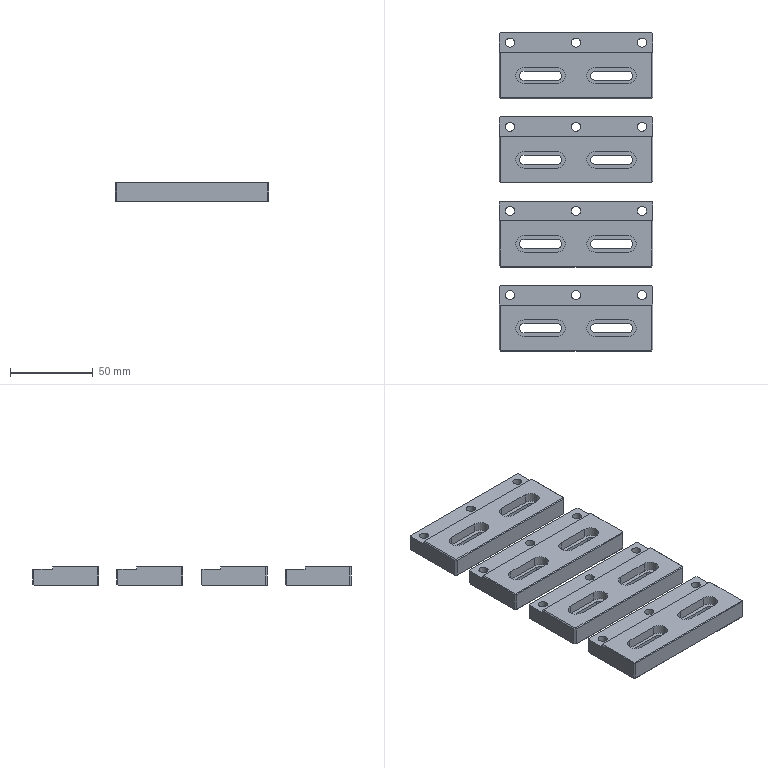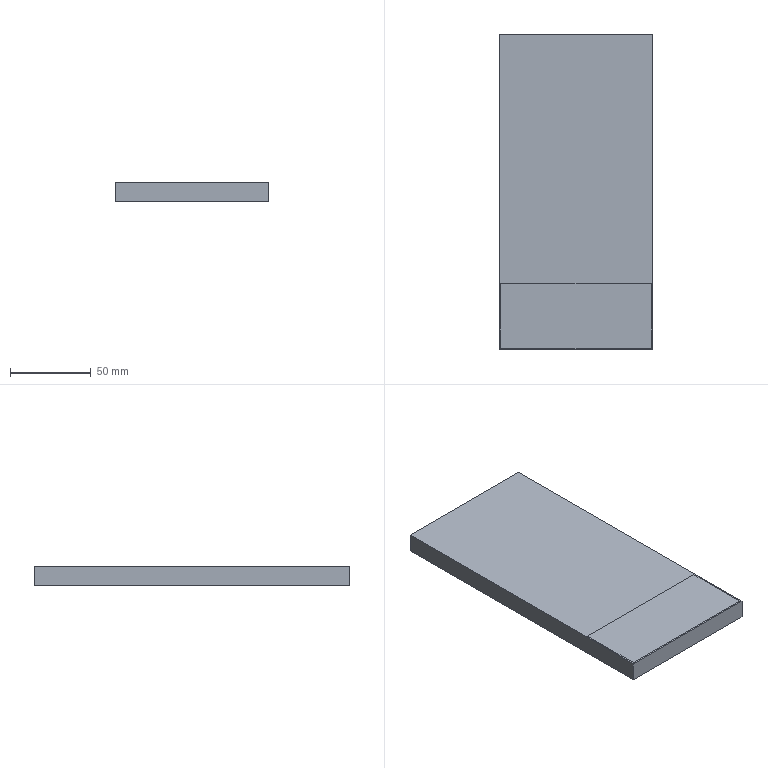CAM job | NX | 3-axis milling, drilling | part box 93.002 x 193 x 12 mm | stock box 95.002 x 195 x 12 mm
Tools:
number,name,description,diameter,corner_radius,flute_length,length,flutes
1,ZXZ,Milling Tool-5 Parameters,6.0,0.0,50.0,75.0,2
6,D6,Milling Tool-5 Parameters,6.0,0.0,50.0,75.0,2
22,D6A45,Milling Tool-5 Parameters,6.0,0.0,3.0,3.0,2
7,D6JING,Milling Tool-5 Parameters,6.0,0.0,50.0,75.0,2
10,D10,Milling Tool-5 Parameters,10.0,0.0,50.0,75.0,2
4,D4,Milling Tool-5 Parameters,4.0,0.0,50.0,75.0,2
11,D10JING,Milling Tool-5 Parameters,10.0,0.0,50.0,75.0,2
15,5.5ZT,Drilling Tool,5.5,0.0,35.0,50.0,2
Operations:
program,operation,operation_type,tool,method,geometry_group,spindle_rpm,surface_speed,feed_per_tooth,feed_cut,feed_plunge,cut_length_mm,path_length_mm,cut_time_min,machine_time_min
1吸-94-194-12毛胚,ZLEVEL_PROFILE,ZLevelMilling,D10,METHOD,A,3500.0,87.0,0.2857,2000.0,100.0,71291.369,71854.751,35.646,35.702
1吸-94-194-12毛胚,FLOOR_WALL,VolumeBased25DMillingOperation,D10,METHOD,A,2500.0,78.0,0.4,2000.0,1000.0,7813.004,8395.277,4.06,4.118
1吸-94-194-12毛胚,DRILLING_COPY_1_COPY_1,Operation,ZXZ,METHOD,A,5000.0,94.0,0.025,250.0,0.0,48.0,667.163,0.192,0.2539
1吸-94-194-12毛胚,DRILLING_COPY_1_COPY_1_COPY,Operation,5.5ZT,METHOD,A,2000.0,31.0,0.0375,150.0,0.0,153.6,878.363,1.024,1.097
1吸-94-194-12毛胚,ZLEVEL_PROFILE_COPY,ZLevelMilling,D6,METHOD,A,4500.0,84.0,0.1667,1500.0,100.0,24129.805,24948.559,16.087,16.168
1吸-94-194-12毛胚,ZLEVEL_PROFILE_COPY_COPY_1,ZLevelMilling,D4,METHOD,A,5500.0,69.0,0.1136,1250.0,100.0,27851.558,28787.664,22.281,22.375
1吸-94-194-12毛胚,ZLEVEL_PROFILE_1_COPY_COPY,ZLevelMilling,D10JING,METHOD,A,7500.0,141.0,0.0833,1250.0,100.0,1223.729,1980.749,0.979,1.055
1吸-94-194-12毛胚,FLOOR_WALL_1_1_COPY,VolumeBased25DMillingOperation,D10JING,METHOD,A,7000.0,219.0,0.0714,1000.0,100.0,1706.188,2980.076,1.706,1.834
1吸-94-194-12毛胚,刀补7_1,VolumeBased25DMillingOperation,D6JING,METHOD,A,7000.0,219.0,0.0714,1000.0,100.0,453.744,1357.813,0.4537,0.5442
1吸-94-194-12毛胚,ZLEVEL_PROFILE_1_COPY_1_COPY,ZLevelMilling,D6A45,METHOD,A,7500.0,141.0,0.0667,1000.0,100.0,1565.649,3027.904,1.566,1.712
1吸-94-194-12毛胚,ZLEVEL_PROFILE_1_COPY_1_COPY_COPY,ZLevelMilling,D6A45,METHOD,A,7500.0,141.0,0.0667,1000.0,100.0,671.634,2644.623,0.6716,0.8689
2虎钳,HOLE_MILLING,CylinderMilling,D6,METHOD,B,4000.0,75.0,0.1812,1450.0,100.0,2393.968,2669.568,1.651,1.679
2虎钳,ZLEVEL_PROFILE_1_COPY_1_COPY_1,ZLevelMilling,D6A45,METHOD,B,7500.0,141.0,0.0667,1000.0,100.0,478.388,1083.34,0.4784,0.5389